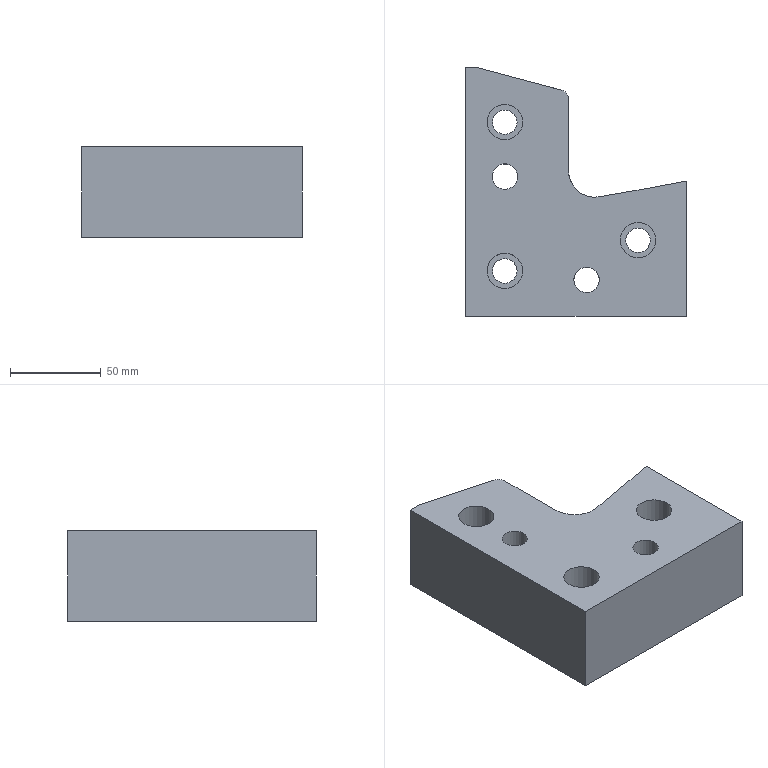Part | NX | features solid 2 | 1 solid | 23 faces | box 121.642 x 136.888 x 50 mm | volume 539772 mm3 | plane 11 | cylinder 10 | spline 2 | commonest cylinder face diameters 13.5 x3 19.5 x3 10 x2 14 x2
STEP:
#1=CARTESIAN_POINT('',(-1318.358,395.,0.));
#2=VERTEX_POINT('',#1);
#3=CARTESIAN_POINT('',(-1325.,395.,0.));
#4=VERTEX_POINT('',#3);
#5=CARTESIAN_POINT('',(-1253.358,395.,0.));
#6=DIRECTION('',(-1.,0.,0.));
#7=VECTOR('',#6,1000.);
#8=LINE('',#5,#7);
#9=EDGE_CURVE('',#2,#4,#8,.T.);
#10=ORIENTED_EDGE('',*,*,#9,.F.);
#11=CARTESIAN_POINT('',(-1318.358,395.,-50.));
#12=VERTEX_POINT('',#11);
#13=CARTESIAN_POINT('',(-1318.358,395.,-15.));
#14=DIRECTION('',(0.,0.,-1.));
#15=VECTOR('',#14,1000.);
#16=LINE('',#13,#15);
#17=EDGE_CURVE('',#2,#12,#16,.T.);
#18=ORIENTED_EDGE('',*,*,#17,.T.);
#19=CARTESIAN_POINT('',(-1325.,395.,-50.));
#20=VERTEX_POINT('',#19);
#21=CARTESIAN_POINT('',(-1021.9,395.,-50.));
#22=DIRECTION('',(1.,0.,0.));
#23=VECTOR('',#22,1000.);
#24=LINE('',#21,#23);
#25=EDGE_CURVE('',#12,#20,#24,.F.);
#26=ORIENTED_EDGE('',*,*,#25,.T.);
#27=CARTESIAN_POINT('',(-1325.,395.,-60.));
#28=DIRECTION('',(0.,0.,-1.));
#29=VECTOR('',#28,1000.);
#30=LINE('',#27,#29);
#31=EDGE_CURVE('',#4,#20,#30,.T.);
#32=ORIENTED_EDGE('',*,*,#31,.F.);
#33=EDGE_LOOP('',(#10,#18,#26,#32));
#34=FACE_BOUND('',#33,.T.);
#35=CARTESIAN_POINT('',(-1245.,395.,0.));
#36=DIRECTION('',(0.,1.,0.));
#37=DIRECTION('',(0.,0.,1.));
#38=AXIS2_PLACEMENT_3D('',#35,#36,#37);
#39=PLANE('',#38);
#40=ADVANCED_FACE('',(#34),#39,.T.);
#41=CARTESIAN_POINT('',(-1310.108,365.,-25.));
#42=VERTEX_POINT('',#41);
#43=CARTESIAN_POINT('',(-1303.358,365.,-25.));
#44=DIRECTION('',(0.,0.,-1.));
#45=DIRECTION('',(-1.,0.,0.));
#46=AXIS2_PLACEMENT_3D('',#43,#44,#45);
#47=CIRCLE('',#46,6.75);
#48=EDGE_CURVE('',#42,#42,#47,.T.);
#49=ORIENTED_EDGE('',*,*,#48,.T.);
#50=EDGE_LOOP('',(#49));
#51=FACE_BOUND('',#50,.T.);
#52=CARTESIAN_POINT('',(-1313.108,365.,-25.));
#53=VERTEX_POINT('',#52);
#54=CARTESIAN_POINT('',(-1303.358,365.,-25.));
#55=DIRECTION('',(0.,0.,-1.));
#56=DIRECTION('',(-1.,0.,0.));
#57=AXIS2_PLACEMENT_3D('',#54,#55,#56);
#58=CIRCLE('',#57,9.75);
#59=EDGE_CURVE('',#53,#53,#58,.T.);
#60=ORIENTED_EDGE('',*,*,#59,.F.);
#61=EDGE_LOOP('',(#60));
#62=FACE_BOUND('',#61,.T.);
#63=CARTESIAN_POINT('',(-1303.358,345.,-25.));
#64=DIRECTION('',(0.,0.,-1.));
#65=DIRECTION('',(-1.,0.,0.));
#66=AXIS2_PLACEMENT_3D('',#63,#64,#65);
#67=PLANE('',#66);
#68=ADVANCED_FACE('',(#51,#62),#67,.F.);
#69=CARTESIAN_POINT('',(-1310.108,283.112,-25.));
#70=VERTEX_POINT('',#69);
#71=CARTESIAN_POINT('',(-1303.358,283.112,-25.));
#72=DIRECTION('',(0.,0.,-1.));
#73=DIRECTION('',(-1.,0.,0.));
#74=AXIS2_PLACEMENT_3D('',#71,#72,#73);
#75=CIRCLE('',#74,6.75);
#76=EDGE_CURVE('',#70,#70,#75,.T.);
#77=ORIENTED_EDGE('',*,*,#76,.T.);
#78=EDGE_LOOP('',(#77));
#79=FACE_BOUND('',#78,.T.);
#80=CARTESIAN_POINT('',(-1313.108,283.112,-25.));
#81=VERTEX_POINT('',#80);
#82=CARTESIAN_POINT('',(-1303.358,283.112,-25.));
#83=DIRECTION('',(0.,0.,-1.));
#84=DIRECTION('',(-1.,0.,0.));
#85=AXIS2_PLACEMENT_3D('',#82,#83,#84);
#86=CIRCLE('',#85,9.75);
#87=EDGE_CURVE('',#81,#81,#86,.T.);
#88=ORIENTED_EDGE('',*,*,#87,.F.);
#89=EDGE_LOOP('',(#88));
#90=FACE_BOUND('',#89,.T.);
#91=CARTESIAN_POINT('',(-1288.358,283.112,-25.));
#92=DIRECTION('',(0.,0.,-1.));
#93=DIRECTION('',(-1.,0.,0.));
#94=AXIS2_PLACEMENT_3D('',#91,#92,#93);
#95=PLANE('',#94);
#96=ADVANCED_FACE('',(#79,#90),#95,.F.);
#97=CARTESIAN_POINT('',(-1236.75,300.,-25.));
#98=VERTEX_POINT('',#97);
#99=CARTESIAN_POINT('',(-1230.,300.,-25.));
#100=DIRECTION('',(0.,0.,-1.));
#101=DIRECTION('',(-1.,0.,0.));
#102=AXIS2_PLACEMENT_3D('',#99,#100,#101);
#103=CIRCLE('',#102,6.75);
#104=EDGE_CURVE('',#98,#98,#103,.T.);
#105=ORIENTED_EDGE('',*,*,#104,.T.);
#106=EDGE_LOOP('',(#105));
#107=FACE_BOUND('',#106,.T.);
#108=CARTESIAN_POINT('',(-1239.75,300.,-25.));
#109=VERTEX_POINT('',#108);
#110=CARTESIAN_POINT('',(-1230.,300.,-25.));
#111=DIRECTION('',(0.,0.,-1.));
#112=DIRECTION('',(-1.,0.,0.));
#113=AXIS2_PLACEMENT_3D('',#110,#111,#112);
#114=CIRCLE('',#113,9.75);
#115=EDGE_CURVE('',#109,#109,#114,.T.);
#116=ORIENTED_EDGE('',*,*,#115,.F.);
#117=EDGE_LOOP('',(#116));
#118=FACE_BOUND('',#117,.T.);
#119=CARTESIAN_POINT('',(-1230.,300.,-25.));
#120=DIRECTION('',(0.,0.,-1.));
#121=DIRECTION('',(-1.,0.,0.));
#122=AXIS2_PLACEMENT_3D('',#119,#120,#121);
#123=PLANE('',#122);
#124=ADVANCED_FACE('',(#107,#118),#123,.F.);
#125=CARTESIAN_POINT('',(-1310.108,365.,-50.));
#126=VERTEX_POINT('',#125);
#127=CARTESIAN_POINT('',(-1303.358,365.,-50.));
#128=DIRECTION('',(0.,0.,-1.));
#129=DIRECTION('',(-1.,0.,0.));
#130=AXIS2_PLACEMENT_3D('',#127,#128,#129);
#131=CIRCLE('',#130,6.75);
#132=EDGE_CURVE('',#126,#126,#131,.T.);
#133=ORIENTED_EDGE('',*,*,#132,.T.);
#134=EDGE_LOOP('',(#133));
#135=FACE_BOUND('',#134,.T.);
#136=ORIENTED_EDGE('',*,*,#48,.F.);
#137=EDGE_LOOP('',(#136));
#138=FACE_BOUND('',#137,.T.);
#139=CARTESIAN_POINT('',(-1303.358,365.,-50.));
#140=DIRECTION('',(0.,0.,-1.));
#141=DIRECTION('',(-1.,0.,0.));
#142=AXIS2_PLACEMENT_3D('',#139,#140,#141);
#143=CYLINDRICAL_SURFACE('',#142,6.75);
#144=ADVANCED_FACE('',(#135,#138),#143,.F.);
#145=CARTESIAN_POINT('',(-1310.108,283.112,-50.));
#146=VERTEX_POINT('',#145);
#147=CARTESIAN_POINT('',(-1303.358,283.112,-50.));
#148=DIRECTION('',(0.,0.,-1.));
#149=DIRECTION('',(-1.,0.,0.));
#150=AXIS2_PLACEMENT_3D('',#147,#148,#149);
#151=CIRCLE('',#150,6.75);
#152=EDGE_CURVE('',#146,#146,#151,.T.);
#153=ORIENTED_EDGE('',*,*,#152,.T.);
#154=EDGE_LOOP('',(#153));
#155=FACE_BOUND('',#154,.T.);
#156=ORIENTED_EDGE('',*,*,#76,.F.);
#157=EDGE_LOOP('',(#156));
#158=FACE_BOUND('',#157,.T.);
#159=CARTESIAN_POINT('',(-1303.358,283.112,-50.));
#160=DIRECTION('',(0.,0.,-1.));
#161=DIRECTION('',(-1.,0.,0.));
#162=AXIS2_PLACEMENT_3D('',#159,#160,#161);
#163=CYLINDRICAL_SURFACE('',#162,6.75);
#164=ADVANCED_FACE('',(#155,#158),#163,.F.);
#165=CARTESIAN_POINT('',(-1236.75,300.,-50.));
#166=VERTEX_POINT('',#165);
#167=CARTESIAN_POINT('',(-1230.,300.,-50.));
#168=DIRECTION('',(0.,0.,-1.));
#169=DIRECTION('',(-1.,0.,0.));
#170=AXIS2_PLACEMENT_3D('',#167,#168,#169);
#171=CIRCLE('',#170,6.75);
#172=EDGE_CURVE('',#166,#166,#171,.T.);
#173=ORIENTED_EDGE('',*,*,#172,.T.);
#174=EDGE_LOOP('',(#173));
#175=FACE_BOUND('',#174,.T.);
#176=ORIENTED_EDGE('',*,*,#104,.F.);
#177=EDGE_LOOP('',(#176));
#178=FACE_BOUND('',#177,.T.);
#179=CARTESIAN_POINT('',(-1230.,300.,-50.));
#180=DIRECTION('',(0.,0.,-1.));
#181=DIRECTION('',(-1.,0.,0.));
#182=AXIS2_PLACEMENT_3D('',#179,#180,#181);
#183=CYLINDRICAL_SURFACE('',#182,6.75);
#184=ADVANCED_FACE('',(#175,#178),#183,.F.);
#185=CARTESIAN_POINT('',(-1203.358,258.112,-50.));
#186=VERTEX_POINT('',#185);
#187=CARTESIAN_POINT('',(-1203.358,258.112,0.));
#188=VERTEX_POINT('',#187);
#189=CARTESIAN_POINT('',(-1203.358,258.112,-50.));
#190=DIRECTION('',(0.,0.,1.));
#191=VECTOR('',#190,1000.);
#192=LINE('',#189,#191);
#193=EDGE_CURVE('',#186,#188,#192,.T.);
#194=ORIENTED_EDGE('',*,*,#193,.T.);
#195=CARTESIAN_POINT('',(-1325.,258.112,0.));
#196=VERTEX_POINT('',#195);
#197=CARTESIAN_POINT('',(-1253.358,258.112,0.));
#198=DIRECTION('',(-1.,0.,0.));
#199=VECTOR('',#198,1000.);
#200=LINE('',#197,#199);
#201=EDGE_CURVE('',#188,#196,#200,.T.);
#202=ORIENTED_EDGE('',*,*,#201,.T.);
#203=CARTESIAN_POINT('',(-1325.,258.112,-50.));
#204=VERTEX_POINT('',#203);
#205=CARTESIAN_POINT('',(-1325.,258.112,-60.));
#206=DIRECTION('',(0.,0.,-1.));
#207=VECTOR('',#206,1000.);
#208=LINE('',#205,#207);
#209=EDGE_CURVE('',#196,#204,#208,.T.);
#210=ORIENTED_EDGE('',*,*,#209,.T.);
#211=CARTESIAN_POINT('',(-1021.9,258.112,-50.));
#212=DIRECTION('',(1.,0.,0.));
#213=VECTOR('',#212,1000.);
#214=LINE('',#211,#213);
#215=EDGE_CURVE('',#186,#204,#214,.F.);
#216=ORIENTED_EDGE('',*,*,#215,.F.);
#217=EDGE_LOOP('',(#194,#202,#210,#216));
#218=FACE_BOUND('',#217,.T.);
#219=CARTESIAN_POINT('',(-1203.358,258.112,0.));
#220=DIRECTION('',(0.,1.,0.));
#221=DIRECTION('',(0.,0.,1.));
#222=AXIS2_PLACEMENT_3D('',#219,#220,#221);
#223=PLANE('',#222);
#224=ADVANCED_FACE('',(#218),#223,.F.);
#225=CARTESIAN_POINT('',(-1265.358,278.112,-50.));
#226=VERTEX_POINT('',#225);
#227=CARTESIAN_POINT('',(-1258.358,278.112,-50.));
#228=DIRECTION('',(0.,0.,-1.));
#229=DIRECTION('',(-1.,0.,0.));
#230=AXIS2_PLACEMENT_3D('',#227,#228,#229);
#231=CIRCLE('',#230,7.);
#232=EDGE_CURVE('',#226,#226,#231,.T.);
#233=ORIENTED_EDGE('',*,*,#232,.T.);
#234=EDGE_LOOP('',(#233));
#235=FACE_BOUND('',#234,.T.);
#236=CARTESIAN_POINT('',(-1265.358,278.112,0.));
#237=VERTEX_POINT('',#236);
#238=CARTESIAN_POINT('',(-1258.358,278.112,0.));
#239=DIRECTION('',(0.,0.,-1.));
#240=DIRECTION('',(-1.,0.,0.));
#241=AXIS2_PLACEMENT_3D('',#238,#239,#240);
#242=CIRCLE('',#241,7.);
#243=EDGE_CURVE('',#237,#237,#242,.T.);
#244=ORIENTED_EDGE('',*,*,#243,.F.);
#245=EDGE_LOOP('',(#244));
#246=FACE_BOUND('',#245,.T.);
#247=CARTESIAN_POINT('',(-1258.358,278.112,0.));
#248=DIRECTION('',(0.,0.,-1.));
#249=DIRECTION('',(-1.,0.,0.));
#250=AXIS2_PLACEMENT_3D('',#247,#248,#249);
#251=CYLINDRICAL_SURFACE('',#250,7.);
#252=ADVANCED_FACE('',(#235,#246),#251,.F.);
#253=ORIENTED_EDGE('',*,*,#59,.T.);
#254=EDGE_LOOP('',(#253));
#255=FACE_BOUND('',#254,.T.);
#256=CARTESIAN_POINT('',(-1313.108,365.,0.));
#257=VERTEX_POINT('',#256);
#258=CARTESIAN_POINT('',(-1303.358,365.,0.));
#259=DIRECTION('',(0.,0.,-1.));
#260=DIRECTION('',(-1.,0.,0.));
#261=AXIS2_PLACEMENT_3D('',#258,#259,#260);
#262=CIRCLE('',#261,9.75);
#263=EDGE_CURVE('',#257,#257,#262,.T.);
#264=ORIENTED_EDGE('',*,*,#263,.F.);
#265=EDGE_LOOP('',(#264));
#266=FACE_BOUND('',#265,.T.);
#267=CARTESIAN_POINT('',(-1303.358,365.,0.));
#268=DIRECTION('',(0.,0.,-1.));
#269=DIRECTION('',(-1.,0.,0.));
#270=AXIS2_PLACEMENT_3D('',#267,#268,#269);
#271=CYLINDRICAL_SURFACE('',#270,9.75);
#272=ADVANCED_FACE('',(#255,#266),#271,.F.);
#273=ORIENTED_EDGE('',*,*,#87,.T.);
#274=EDGE_LOOP('',(#273));
#275=FACE_BOUND('',#274,.T.);
#276=CARTESIAN_POINT('',(-1313.108,283.112,0.));
#277=VERTEX_POINT('',#276);
#278=CARTESIAN_POINT('',(-1303.358,283.112,0.));
#279=DIRECTION('',(0.,0.,-1.));
#280=DIRECTION('',(-1.,0.,0.));
#281=AXIS2_PLACEMENT_3D('',#278,#279,#280);
#282=CIRCLE('',#281,9.75);
#283=EDGE_CURVE('',#277,#277,#282,.T.);
#284=ORIENTED_EDGE('',*,*,#283,.F.);
#285=EDGE_LOOP('',(#284));
#286=FACE_BOUND('',#285,.T.);
#287=CARTESIAN_POINT('',(-1303.358,283.112,0.));
#288=DIRECTION('',(0.,0.,-1.));
#289=DIRECTION('',(-1.,0.,0.));
#290=AXIS2_PLACEMENT_3D('',#287,#288,#289);
#291=CYLINDRICAL_SURFACE('',#290,9.75);
#292=ADVANCED_FACE('',(#275,#286),#291,.F.);
#293=ORIENTED_EDGE('',*,*,#115,.T.);
#294=EDGE_LOOP('',(#293));
#295=FACE_BOUND('',#294,.T.);
#296=CARTESIAN_POINT('',(-1239.75,300.,0.));
#297=VERTEX_POINT('',#296);
#298=CARTESIAN_POINT('',(-1230.,300.,0.));
#299=DIRECTION('',(0.,0.,-1.));
#300=DIRECTION('',(-1.,0.,0.));
#301=AXIS2_PLACEMENT_3D('',#298,#299,#300);
#302=CIRCLE('',#301,9.75);
#303=EDGE_CURVE('',#297,#297,#302,.T.);
#304=ORIENTED_EDGE('',*,*,#303,.F.);
#305=EDGE_LOOP('',(#304));
#306=FACE_BOUND('',#305,.T.);
#307=CARTESIAN_POINT('',(-1230.,300.,0.));
#308=DIRECTION('',(0.,0.,-1.));
#309=DIRECTION('',(-1.,0.,0.));
#310=AXIS2_PLACEMENT_3D('',#307,#308,#309);
#311=CYLINDRICAL_SURFACE('',#310,9.75);
#312=ADVANCED_FACE('',(#295,#306),#311,.F.);
#313=CARTESIAN_POINT('',(-1203.358,332.538,-15.));
#314=VERTEX_POINT('',#313);
#315=CARTESIAN_POINT('',(-1203.358,330.489,-15.));
#316=VERTEX_POINT('',#315);
#317=CARTESIAN_POINT('',(-1203.358,250.,-15.));
#318=DIRECTION('',(0.,1.,0.));
#319=VECTOR('',#318,1000.);
#320=LINE('',#317,#319);
#321=EDGE_CURVE('',#314,#316,#320,.F.);
#322=ORIENTED_EDGE('',*,*,#321,.F.);
#323=CARTESIAN_POINT('',(-1203.358,332.538,0.));
#324=VERTEX_POINT('',#323);
#325=CARTESIAN_POINT('',(-1203.358,332.538,-100.));
#326=DIRECTION('',(0.,0.,1.));
#327=VECTOR('',#326,1000.);
#328=LINE('',#325,#327);
#329=EDGE_CURVE('',#324,#314,#328,.F.);
#330=ORIENTED_EDGE('',*,*,#329,.F.);
#331=CARTESIAN_POINT('',(-1203.358,307.899,0.));
#332=DIRECTION('',(0.,-1.,0.));
#333=VECTOR('',#332,1000.);
#334=LINE('',#331,#333);
#335=EDGE_CURVE('',#324,#188,#334,.T.);
#336=ORIENTED_EDGE('',*,*,#335,.T.);
#337=ORIENTED_EDGE('',*,*,#193,.F.);
#338=CARTESIAN_POINT('',(-1203.358,330.489,-50.));
#339=VERTEX_POINT('',#338);
#340=CARTESIAN_POINT('',(-1203.358,307.899,-50.));
#341=DIRECTION('',(0.,-1.,0.));
#342=VECTOR('',#341,1000.);
#343=LINE('',#340,#342);
#344=EDGE_CURVE('',#339,#186,#343,.T.);
#345=ORIENTED_EDGE('',*,*,#344,.F.);
#346=CARTESIAN_POINT('',(-1203.358,330.489,-32.5));
#347=DIRECTION('',(0.,0.,1.));
#348=VECTOR('',#347,1000.);
#349=LINE('',#346,#348);
#350=EDGE_CURVE('',#339,#316,#349,.T.);
#351=ORIENTED_EDGE('',*,*,#350,.T.);
#352=EDGE_LOOP('',(#322,#330,#336,#337,#345,#351));
#353=FACE_BOUND('',#352,.T.);
#354=CARTESIAN_POINT('',(-1203.358,250.,0.));
#355=DIRECTION('',(1.,0.,0.));
#356=DIRECTION('',(0.,0.,-1.));
#357=AXIS2_PLACEMENT_3D('',#354,#355,#356);
#358=PLANE('',#357);
#359=ADVANCED_FACE('',(#353),#358,.T.);
#360=CARTESIAN_POINT('',(-1270.358,378.302,-50.));
#361=VERTEX_POINT('',#360);
#362=CARTESIAN_POINT('',(-1203.358,330.489,-50.));
#363=CARTESIAN_POINT('',(-1208.021,329.456,-50.));
#364=CARTESIAN_POINT('',(-1215.042,328.141,-50.));
#365=CARTESIAN_POINT('',(-1224.396,326.524,-50.));
#366=CARTESIAN_POINT('',(-1231.398,325.331,-50.));
#367=CARTESIAN_POINT('',(-1237.23,324.32,-50.));
#368=CARTESIAN_POINT('',(-1241.899,323.51,-50.));
#369=CARTESIAN_POINT('',(-1245.394,322.899,-50.));
#370=CARTESIAN_POINT('',(-1248.327,322.398,-50.));
#371=CARTESIAN_POINT('',(-1250.62,321.979,-50.));
#372=CARTESIAN_POINT('',(-1252.531,321.673,-50.));
#373=CARTESIAN_POINT('',(-1254.609,321.607,-50.));
#374=CARTESIAN_POINT('',(-1257.298,321.883,-50.));
#375=CARTESIAN_POINT('',(-1260.584,322.891,-50.));
#376=CARTESIAN_POINT('',(-1264.046,325.04,-50.));
#377=CARTESIAN_POINT('',(-1266.887,327.947,-50.));
#378=CARTESIAN_POINT('',(-1268.96,331.413,-50.));
#379=CARTESIAN_POINT('',(-1270.19,335.291,-50.));
#380=CARTESIAN_POINT('',(-1270.428,339.274,-50.));
#381=CARTESIAN_POINT('',(-1270.366,342.757,-50.));
#382=CARTESIAN_POINT('',(-1270.377,346.328,-50.));
#383=CARTESIAN_POINT('',(-1270.367,351.059,-50.));
#384=CARTESIAN_POINT('',(-1270.365,356.984,-50.));
#385=CARTESIAN_POINT('',(-1270.36,364.089,-50.));
#386=CARTESIAN_POINT('',(-1270.359,371.195,-50.));
#387=CARTESIAN_POINT('',(-1270.358,375.933,-50.));
#388=CARTESIAN_POINT('',(-1270.358,378.302,-50.));
#389=B_SPLINE_CURVE_WITH_KNOTS('',3,(#362,#363,#364,#365,#366,#367,#368,#369,#370,#371,#372,#373,#374,#375,#376,#377,#378,#379,#380,#381,#382,#383,#384,#385,#386,#387,#388),.UNSPECIFIED.,.F.,.F.,(4,1,1,1,1,1,1,1,1,1,1,1,1,1,1,1,1,1,1,1,1,1,1,1,4),(0.002675,0.08837,0.1312,0.1741,0.2169,0.2383,0.2598,0.2812,0.2919,0.3026,0.3133,0.324,0.3455,0.3669,0.3883,0.4097,0.4312,0.4526,0.474,0.4954,0.5169,0.5597,0.6026,0.6454,0.6883),.UNSPECIFIED.);
#390=EDGE_CURVE('',#339,#361,#389,.T.);
#391=ORIENTED_EDGE('',*,*,#390,.T.);
#392=CARTESIAN_POINT('',(-1270.358,378.302,-15.));
#393=VERTEX_POINT('',#392);
#394=CARTESIAN_POINT('',(-1270.358,378.302,-15.));
#395=CARTESIAN_POINT('',(-1270.358,378.302,-26.667));
#396=CARTESIAN_POINT('',(-1270.358,378.302,-38.333));
#397=CARTESIAN_POINT('',(-1270.358,378.302,-50.));
#398=B_SPLINE_CURVE_WITH_KNOTS('',3,(#394,#395,#396,#397),.UNSPECIFIED.,.F.,.F.,(4,4),(0.,1.),.UNSPECIFIED.);
#399=EDGE_CURVE('',#361,#393,#398,.F.);
#400=ORIENTED_EDGE('',*,*,#399,.T.);
#401=CARTESIAN_POINT('',(-1203.358,330.489,-15.));
#402=CARTESIAN_POINT('',(-1208.021,329.456,-15.));
#403=CARTESIAN_POINT('',(-1215.042,328.141,-15.));
#404=CARTESIAN_POINT('',(-1224.396,326.524,-15.));
#405=CARTESIAN_POINT('',(-1231.398,325.331,-15.));
#406=CARTESIAN_POINT('',(-1237.23,324.32,-15.));
#407=CARTESIAN_POINT('',(-1241.899,323.51,-15.));
#408=CARTESIAN_POINT('',(-1245.394,322.899,-15.));
#409=CARTESIAN_POINT('',(-1248.327,322.398,-15.));
#410=CARTESIAN_POINT('',(-1250.62,321.979,-15.));
#411=CARTESIAN_POINT('',(-1252.531,321.673,-15.));
#412=CARTESIAN_POINT('',(-1254.609,321.607,-15.));
#413=CARTESIAN_POINT('',(-1257.298,321.883,-15.));
#414=CARTESIAN_POINT('',(-1260.584,322.891,-15.));
#415=CARTESIAN_POINT('',(-1264.046,325.04,-15.));
#416=CARTESIAN_POINT('',(-1266.887,327.947,-15.));
#417=CARTESIAN_POINT('',(-1268.96,331.413,-15.));
#418=CARTESIAN_POINT('',(-1270.19,335.291,-15.));
#419=CARTESIAN_POINT('',(-1270.428,339.274,-15.));
#420=CARTESIAN_POINT('',(-1270.366,342.757,-15.));
#421=CARTESIAN_POINT('',(-1270.377,346.328,-15.));
#422=CARTESIAN_POINT('',(-1270.367,351.059,-15.));
#423=CARTESIAN_POINT('',(-1270.365,356.984,-15.));
#424=CARTESIAN_POINT('',(-1270.36,364.089,-15.));
#425=CARTESIAN_POINT('',(-1270.359,371.195,-15.));
#426=CARTESIAN_POINT('',(-1270.358,375.933,-15.));
#427=CARTESIAN_POINT('',(-1270.358,378.302,-15.));
#428=B_SPLINE_CURVE_WITH_KNOTS('',3,(#401,#402,#403,#404,#405,#406,#407,#408,#409,#410,#411,#412,#413,#414,#415,#416,#417,#418,#419,#420,#421,#422,#423,#424,#425,#426,#427),.UNSPECIFIED.,.F.,.F.,(4,1,1,1,1,1,1,1,1,1,1,1,1,1,1,1,1,1,1,1,1,1,1,1,4),(0.002675,0.08837,0.1312,0.1741,0.2169,0.2383,0.2598,0.2812,0.2919,0.3026,0.3133,0.324,0.3455,0.3669,0.3883,0.4097,0.4312,0.4526,0.474,0.4954,0.5169,0.5597,0.6026,0.6454,0.6883),.UNSPECIFIED.);
#429=EDGE_CURVE('',#316,#393,#428,.T.);
#430=ORIENTED_EDGE('',*,*,#429,.F.);
#431=ORIENTED_EDGE('',*,*,#350,.F.);
#432=EDGE_LOOP('',(#391,#400,#430,#431));
#433=FACE_BOUND('',#432,.T.);
#434=CARTESIAN_POINT('',(-1203.358,330.489,-50.));
#435=CARTESIAN_POINT('',(-1203.358,330.489,-15.));
#436=CARTESIAN_POINT('',(-1208.021,329.456,-50.));
#437=CARTESIAN_POINT('',(-1208.021,329.456,-15.));
#438=CARTESIAN_POINT('',(-1215.042,328.141,-50.));
#439=CARTESIAN_POINT('',(-1215.042,328.141,-15.));
#440=CARTESIAN_POINT('',(-1224.396,326.524,-50.));
#441=CARTESIAN_POINT('',(-1224.396,326.524,-15.));
#442=CARTESIAN_POINT('',(-1231.398,325.331,-50.));
#443=CARTESIAN_POINT('',(-1231.398,325.331,-15.));
#444=CARTESIAN_POINT('',(-1237.23,324.32,-50.));
#445=CARTESIAN_POINT('',(-1237.23,324.32,-15.));
#446=CARTESIAN_POINT('',(-1241.899,323.51,-50.));
#447=CARTESIAN_POINT('',(-1241.899,323.51,-15.));
#448=CARTESIAN_POINT('',(-1245.394,322.899,-50.));
#449=CARTESIAN_POINT('',(-1245.394,322.899,-15.));
#450=CARTESIAN_POINT('',(-1248.327,322.398,-50.));
#451=CARTESIAN_POINT('',(-1248.327,322.398,-15.));
#452=CARTESIAN_POINT('',(-1250.62,321.979,-50.));
#453=CARTESIAN_POINT('',(-1250.62,321.979,-15.));
#454=CARTESIAN_POINT('',(-1252.531,321.673,-50.));
#455=CARTESIAN_POINT('',(-1252.531,321.673,-15.));
#456=CARTESIAN_POINT('',(-1254.609,321.607,-50.));
#457=CARTESIAN_POINT('',(-1254.609,321.607,-15.));
#458=CARTESIAN_POINT('',(-1257.298,321.883,-50.));
#459=CARTESIAN_POINT('',(-1257.298,321.883,-15.));
#460=CARTESIAN_POINT('',(-1260.584,322.891,-50.));
#461=CARTESIAN_POINT('',(-1260.584,322.891,-15.));
#462=CARTESIAN_POINT('',(-1264.046,325.04,-50.));
#463=CARTESIAN_POINT('',(-1264.046,325.04,-15.));
#464=CARTESIAN_POINT('',(-1266.887,327.947,-50.));
#465=CARTESIAN_POINT('',(-1266.887,327.947,-15.));
#466=CARTESIAN_POINT('',(-1268.96,331.413,-50.));
#467=CARTESIAN_POINT('',(-1268.96,331.413,-15.));
#468=CARTESIAN_POINT('',(-1270.19,335.291,-50.));
#469=CARTESIAN_POINT('',(-1270.19,335.291,-15.));
#470=CARTESIAN_POINT('',(-1270.428,339.274,-50.));
#471=CARTESIAN_POINT('',(-1270.428,339.274,-15.));
#472=CARTESIAN_POINT('',(-1270.366,342.757,-50.));
#473=CARTESIAN_POINT('',(-1270.366,342.757,-15.));
#474=CARTESIAN_POINT('',(-1270.377,346.328,-50.));
#475=CARTESIAN_POINT('',(-1270.377,346.328,-15.));
#476=CARTESIAN_POINT('',(-1270.367,351.059,-50.));
#477=CARTESIAN_POINT('',(-1270.367,351.059,-15.));
#478=CARTESIAN_POINT('',(-1270.365,356.984,-50.));
#479=CARTESIAN_POINT('',(-1270.365,356.984,-15.));
#480=CARTESIAN_POINT('',(-1270.36,364.089,-50.));
#481=CARTESIAN_POINT('',(-1270.36,364.089,-15.));
#482=CARTESIAN_POINT('',(-1270.359,371.195,-50.));
#483=CARTESIAN_POINT('',(-1270.359,371.195,-15.));
#484=CARTESIAN_POINT('',(-1270.358,375.933,-50.));
#485=CARTESIAN_POINT('',(-1270.358,375.933,-15.));
#486=CARTESIAN_POINT('',(-1270.358,378.302,-50.));
#487=CARTESIAN_POINT('',(-1270.358,378.302,-15.));
#488=B_SPLINE_SURFACE_WITH_KNOTS('',3,1,((#434,#435),(#436,#437),(#438,#439),(#440,#441),(#442,#443),(#444,#445),(#446,#447),(#448,#449),(#450,#451),(#452,#453),(#454,#455),(#456,#457),(#458,#459),(#460,#461),(#462,#463),(#464,#465),(#466,#467),(#468,#469),(#470,#471),(#472,#473),(#474,#475),(#476,#477),(#478,#479),(#480,#481),(#482,#483),(#484,#485),(#486,#487)),.SURF_OF_LINEAR_EXTRUSION.,.F.,.F.,.F.,(4,1,1,1,1,1,1,1,1,1,1,1,1,1,1,1,1,1,1,1,1,1,1,1,4),(2,2),(0.002675,0.08837,0.1312,0.1741,0.2169,0.2383,0.2598,0.2812,0.2919,0.3026,0.3133,0.324,0.3455,0.3669,0.3883,0.4097,0.4312,0.4526,0.474,0.4954,0.5169,0.5597,0.6026,0.6454,0.6883),(0.,1.),.UNSPECIFIED.);
#489=ADVANCED_FACE('',(#433),#488,.T.);
#490=CARTESIAN_POINT('',(-1274.064,383.131,-15.));
#491=VERTEX_POINT('',#490);
#492=CARTESIAN_POINT('',(-1272.064,382.595,-15.));
#493=VERTEX_POINT('',#492);
#494=CARTESIAN_POINT('',(-1318.358,395.,-15.));
#495=DIRECTION('',(-0.9659,0.2588,0.));
#496=VECTOR('',#495,1000.);
#497=LINE('',#494,#496);
#498=EDGE_CURVE('',#491,#493,#497,.F.);
#499=ORIENTED_EDGE('',*,*,#498,.T.);
#500=CARTESIAN_POINT('',(-1268.358,377.766,-15.));
#501=VERTEX_POINT('',#500);
#502=CARTESIAN_POINT('',(-1273.358,377.766,-15.));
#503=DIRECTION('',(0.,0.,-1.));
#504=DIRECTION('',(-1.,0.,0.));
#505=AXIS2_PLACEMENT_3D('',#502,#503,#504);
#506=CIRCLE('',#505,5.);
#507=EDGE_CURVE('',#493,#501,#506,.T.);
#508=ORIENTED_EDGE('',*,*,#507,.T.);
#509=CARTESIAN_POINT('',(-169.554,563.744,-15.));
#510=CARTESIAN_POINT('',(-255.297,544.568,-15.));
#511=CARTESIAN_POINT('',(-341.04,525.392,-15.));
#512=CARTESIAN_POINT('',(-426.783,506.216,-15.));
#513=CARTESIAN_POINT('',(-492.739,491.465,-15.));
#514=CARTESIAN_POINT('',(-558.696,476.715,-15.));
#515=CARTESIAN_POINT('',(-624.652,461.964,-15.));
#516=CARTESIAN_POINT('',(-675.387,450.617,-15.));
#517=CARTESIAN_POINT('',(-726.123,439.27,-15.));
#518=CARTESIAN_POINT('',(-776.858,427.923,-15.));
#519=CARTESIAN_POINT('',(-815.885,419.195,-15.));
#520=CARTESIAN_POINT('',(-854.913,410.467,-15.));
#521=CARTESIAN_POINT('',(-893.94,401.738,-15.));
#522=CARTESIAN_POINT('',(-923.961,395.024,-15.));
#523=CARTESIAN_POINT('',(-953.982,388.31,-15.));
#524=CARTESIAN_POINT('',(-984.003,381.596,-15.));
#525=CARTESIAN_POINT('',(-1007.096,376.432,-15.));
#526=CARTESIAN_POINT('',(-1030.189,371.267,-15.));
#527=CARTESIAN_POINT('',(-1053.282,366.102,-15.));
#528=CARTESIAN_POINT('',(-1071.046,362.129,-15.));
#529=CARTESIAN_POINT('',(-1088.81,358.157,-15.));
#530=CARTESIAN_POINT('',(-1106.574,354.184,-15.));
#531=CARTESIAN_POINT('',(-1120.238,351.128,-15.));
#532=CARTESIAN_POINT('',(-1133.903,348.072,-15.));
#533=CARTESIAN_POINT('',(-1147.568,345.016,-15.));
#534=CARTESIAN_POINT('',(-1158.079,342.665,-15.));
#535=CARTESIAN_POINT('',(-1168.59,340.314,-15.));
#536=CARTESIAN_POINT('',(-1179.101,337.963,-15.));
#537=CARTESIAN_POINT('',(-1187.187,336.155,-15.));
#538=CARTESIAN_POINT('',(-1195.272,334.347,-15.));
#539=CARTESIAN_POINT('',(-1203.358,332.538,-15.));
#540=CARTESIAN_POINT('',(-1203.741,332.453,-15.));
#541=CARTESIAN_POINT('',(-1207.014,331.73,-15.));
#542=CARTESIAN_POINT('',(-1215.576,330.046,-15.));
#543=CARTESIAN_POINT('',(-1229.105,327.764,-15.));
#544=CARTESIAN_POINT('',(-1240.809,325.729,-15.));
#545=CARTESIAN_POINT('',(-1247.768,324.519,-15.));
#546=CARTESIAN_POINT('',(-1249.983,324.133,-15.));
#547=CARTESIAN_POINT('',(-1251.61,323.834,-15.));
#548=CARTESIAN_POINT('',(-1253.223,323.633,-15.));
#549=CARTESIAN_POINT('',(-1255.35,323.635,-15.));
#550=CARTESIAN_POINT('',(-1259.031,324.277,-15.));
#551=CARTESIAN_POINT('',(-1263.737,327.014,-15.));
#552=CARTESIAN_POINT('',(-1266.869,331.442,-15.));
#553=CARTESIAN_POINT('',(-1268.142,335.513,-15.));
#554=CARTESIAN_POINT('',(-1268.384,338.163,-15.));
#555=CARTESIAN_POINT('',(-1268.358,356.108,-15.));
#556=CARTESIAN_POINT('',(-1268.358,386.543,-15.));
#557=CARTESIAN_POINT('',(-1268.358,416.449,-15.));
#558=CARTESIAN_POINT('',(-1268.358,430.,-15.));
#559=CARTESIAN_POINT('',(-1268.358,438.292,-15.));
#560=CARTESIAN_POINT('',(-1268.358,446.585,-15.));
#561=CARTESIAN_POINT('',(-1268.358,454.877,-15.));
#562=CARTESIAN_POINT('',(-1268.358,465.657,-15.));
#563=CARTESIAN_POINT('',(-1268.358,476.437,-15.));
#564=CARTESIAN_POINT('',(-1268.358,487.217,-15.));
#565=CARTESIAN_POINT('',(-1268.358,501.231,-15.));
#566=CARTESIAN_POINT('',(-1268.358,515.245,-15.));
#567=CARTESIAN_POINT('',(-1268.358,529.259,-15.));
#568=CARTESIAN_POINT('',(-1268.358,547.477,-15.));
#569=CARTESIAN_POINT('',(-1268.358,565.695,-15.));
#570=CARTESIAN_POINT('',(-1268.358,583.913,-15.));
#571=CARTESIAN_POINT('',(-1268.358,607.597,-15.));
#572=CARTESIAN_POINT('',(-1268.358,631.281,-15.));
#573=CARTESIAN_POINT('',(-1268.358,654.964,-15.));
#574=CARTESIAN_POINT('',(-1268.358,685.753,-15.));
#575=CARTESIAN_POINT('',(-1268.358,716.542,-15.));
#576=CARTESIAN_POINT('',(-1268.358,747.33,-15.));
#577=CARTESIAN_POINT('',(-1268.358,787.356,-15.));
#578=CARTESIAN_POINT('',(-1268.358,827.381,-15.));
#579=CARTESIAN_POINT('',(-1268.358,867.406,-15.));
#580=CARTESIAN_POINT('',(-1268.358,919.439,-15.));
#581=CARTESIAN_POINT('',(-1268.358,971.472,-15.));
#582=CARTESIAN_POINT('',(-1268.358,1023.505,-15.));
#583=CARTESIAN_POINT('',(-1268.358,1091.148,-15.));
#584=CARTESIAN_POINT('',(-1268.358,1158.791,-15.));
#585=CARTESIAN_POINT('',(-1268.358,1226.434,-15.));
#586=CARTESIAN_POINT('',(-1268.358,1314.37,-15.));
#587=CARTESIAN_POINT('',(-1268.358,1402.305,-15.));
#588=CARTESIAN_POINT('',(-1268.358,1490.241,-15.));
#589=B_SPLINE_CURVE_WITH_KNOTS('',3,(#509,#510,#511,#512,#513,#514,#515,#516,#517,#518,#519,#520,#521,#522,#523,#524,#525,#526,#527,#528,#529,#530,#531,#532,#533,#534,#535,#536,#537,#538,#539,#540,#541,#542,#543,#544,#545,#546,#547,#548,#549,#550,#551,#552,#553,#554,#555,#556,#557,#558,#559,#560,#561,#562,#563,#564,#565,#566,#567,#568,#569,#570,#571,#572,#573,#574,#575,#576,#577,#578,#579,#580,#581,#582,#583,#584,#585,#586,#587,#588),.UNSPECIFIED.,.F.,.F.,(4,3,3,3,3,3,3,3,3,3,3,1,1,1,1,1,1,1,1,1,1,1,1,1,1,1,1,3,3,3,3,3,3,3,3,3,3,4),(-6.393,-4.802,-3.579,-2.637,-1.913,-1.356,-0.9281,-0.5985,-0.345,-0.15,0.,0.007116,0.06068,0.158,0.2552,0.2756,0.2857,0.2959,0.3055,0.3151,0.3343,0.3727,0.4111,0.4303,0.4495,0.459,0.7549,1.,1.15,1.345,1.599,1.928,2.356,2.913,3.637,4.579,5.802,7.393),.UNSPECIFIED.);
#590=EDGE_CURVE('',#314,#501,#589,.T.);
#591=ORIENTED_EDGE('',*,*,#590,.F.);
#592=ORIENTED_EDGE('',*,*,#321,.T.);
#593=ORIENTED_EDGE('',*,*,#429,.T.);
#594=CARTESIAN_POINT('',(-1275.358,378.302,-15.));
#595=DIRECTION('',(0.,0.,-1.));
#596=DIRECTION('',(-1.,0.,0.));
#597=AXIS2_PLACEMENT_3D('',#594,#595,#596);
#598=CIRCLE('',#597,5.);
#599=EDGE_CURVE('',#393,#491,#598,.F.);
#600=ORIENTED_EDGE('',*,*,#599,.T.);
#601=EDGE_LOOP('',(#499,#508,#591,#592,#593,#600));
#602=FACE_BOUND('',#601,.T.);
#603=CARTESIAN_POINT('',(-1203.358,332.538,-15.));
#604=DIRECTION('',(0.,0.,-1.));
#605=DIRECTION('',(-1.,0.,0.));
#606=AXIS2_PLACEMENT_3D('',#603,#604,#605);
#607=PLANE('',#606);
#608=ADVANCED_FACE('',(#602),#607,.T.);
#609=CARTESIAN_POINT('',(-1310.358,335.,0.));
#610=VERTEX_POINT('',#609);
#611=CARTESIAN_POINT('',(-1303.358,335.,0.));
#612=DIRECTION('',(0.,0.,-1.));
#613=DIRECTION('',(-1.,0.,0.));
#614=AXIS2_PLACEMENT_3D('',#611,#612,#613);
#615=CIRCLE('',#614,7.);
#616=EDGE_CURVE('',#610,#610,#615,.T.);
#617=ORIENTED_EDGE('',*,*,#616,.T.);
#618=EDGE_LOOP('',(#617));
#619=FACE_BOUND('',#618,.T.);
#620=ORIENTED_EDGE('',*,*,#303,.T.);
#621=EDGE_LOOP('',(#620));
#622=FACE_BOUND('',#621,.T.);
#623=ORIENTED_EDGE('',*,*,#283,.T.);
#624=EDGE_LOOP('',(#623));
#625=FACE_BOUND('',#624,.T.);
#626=ORIENTED_EDGE('',*,*,#263,.T.);
#627=EDGE_LOOP('',(#626));
#628=FACE_BOUND('',#627,.T.);
#629=ORIENTED_EDGE('',*,*,#243,.T.);
#630=EDGE_LOOP('',(#629));
#631=FACE_BOUND('',#630,.T.);
#632=CARTESIAN_POINT('',(-1268.358,377.766,0.));
#633=VERTEX_POINT('',#632);
#634=CARTESIAN_POINT('',(-1268.358,3406.296,0.));
#635=CARTESIAN_POINT('',(-1268.358,3160.274,0.));
#636=CARTESIAN_POINT('',(-1268.358,2914.251,0.));
#637=CARTESIAN_POINT('',(-1268.358,2668.228,0.));
#638=CARTESIAN_POINT('',(-1268.358,2478.98,0.));
#639=CARTESIAN_POINT('',(-1268.358,2289.732,0.));
#640=CARTESIAN_POINT('',(-1268.358,2100.484,0.));
#641=CARTESIAN_POINT('',(-1268.358,1954.908,0.));
#642=CARTESIAN_POINT('',(-1268.358,1809.333,0.));
#643=CARTESIAN_POINT('',(-1268.358,1663.757,0.));
#644=CARTESIAN_POINT('',(-1268.358,1551.776,0.));
#645=CARTESIAN_POINT('',(-1268.358,1439.795,0.));
#646=CARTESIAN_POINT('',(-1268.358,1327.814,0.));
#647=CARTESIAN_POINT('',(-1268.358,1241.674,0.));
#648=CARTESIAN_POINT('',(-1268.358,1155.535,0.));
#649=CARTESIAN_POINT('',(-1268.358,1069.395,0.));
#650=CARTESIAN_POINT('',(-1268.358,1003.134,0.));
#651=CARTESIAN_POINT('',(-1268.358,936.873,0.));
#652=CARTESIAN_POINT('',(-1268.358,870.612,0.));
#653=CARTESIAN_POINT('',(-1268.358,819.642,0.));
#654=CARTESIAN_POINT('',(-1268.358,768.672,0.));
#655=CARTESIAN_POINT('',(-1268.358,717.702,0.));
#656=CARTESIAN_POINT('',(-1268.358,678.494,0.));
#657=CARTESIAN_POINT('',(-1268.358,639.287,0.));
#658=CARTESIAN_POINT('',(-1268.358,600.079,0.));
#659=CARTESIAN_POINT('',(-1268.358,569.919,0.));
#660=CARTESIAN_POINT('',(-1268.358,539.759,0.));
#661=CARTESIAN_POINT('',(-1268.358,509.6,0.));
#662=CARTESIAN_POINT('',(-1268.358,486.4,0.));
#663=CARTESIAN_POINT('',(-1268.358,463.2,0.));
#664=CARTESIAN_POINT('',(-1268.358,440.,0.));
#665=CARTESIAN_POINT('',(-1268.358,423.116,0.));
#666=CARTESIAN_POINT('',(-1268.358,389.876,0.));
#667=CARTESIAN_POINT('',(-1268.358,356.108,0.));
#668=CARTESIAN_POINT('',(-1268.384,338.163,0.));
#669=CARTESIAN_POINT('',(-1268.142,335.513,0.));
#670=CARTESIAN_POINT('',(-1266.869,331.442,0.));
#671=CARTESIAN_POINT('',(-1263.737,327.014,0.));
#672=CARTESIAN_POINT('',(-1259.031,324.277,0.));
#673=CARTESIAN_POINT('',(-1255.35,323.635,0.));
#674=CARTESIAN_POINT('',(-1253.223,323.633,0.));
#675=CARTESIAN_POINT('',(-1251.61,323.834,0.));
#676=CARTESIAN_POINT('',(-1249.983,324.133,0.));
#677=CARTESIAN_POINT('',(-1247.768,324.519,0.));
#678=CARTESIAN_POINT('',(-1240.809,325.729,0.));
#679=CARTESIAN_POINT('',(-1229.105,327.764,0.));
#680=CARTESIAN_POINT('',(-1215.576,330.046,0.));
#681=CARTESIAN_POINT('',(-1198.69,333.366,0.));
#682=CARTESIAN_POINT('',(-1181.579,338.217,0.));
#683=CARTESIAN_POINT('',(-1161.617,343.876,0.));
#684=CARTESIAN_POINT('',(-1147.182,347.09,0.));
#685=CARTESIAN_POINT('',(-1132.006,349.651,0.));
#686=CARTESIAN_POINT('',(-1113.357,352.894,0.));
#687=CARTESIAN_POINT('',(-1078.972,358.874,0.));
#688=CARTESIAN_POINT('',(-1041.673,365.361,0.));
#689=CARTESIAN_POINT('',(-1004.375,371.848,0.));
#690=CARTESIAN_POINT('',(-976.401,376.715,0.));
#691=CARTESIAN_POINT('',(-948.425,381.569,0.));
#692=CARTESIAN_POINT('',(-929.78,384.838,0.));
#693=CARTESIAN_POINT('',(-920.448,386.415,0.));
#694=CARTESIAN_POINT('',(-897.572,390.281,0.));
#695=CARTESIAN_POINT('',(-874.697,394.148,0.));
#696=CARTESIAN_POINT('',(-851.821,398.014,0.));
#697=CARTESIAN_POINT('',(-822.083,403.041,0.));
#698=CARTESIAN_POINT('',(-792.345,408.067,0.));
#699=CARTESIAN_POINT('',(-762.607,413.094,0.));
#700=CARTESIAN_POINT('',(-723.948,419.628,0.));
#701=CARTESIAN_POINT('',(-685.289,426.162,0.));
#702=CARTESIAN_POINT('',(-646.629,432.697,0.));
#703=CARTESIAN_POINT('',(-596.372,441.191,0.));
#704=CARTESIAN_POINT('',(-546.115,449.686,0.));
#705=CARTESIAN_POINT('',(-495.858,458.181,0.));
#706=CARTESIAN_POINT('',(-430.523,469.224,0.));
#707=CARTESIAN_POINT('',(-365.189,480.267,0.));
#708=CARTESIAN_POINT('',(-299.855,491.31,0.));
#709=CARTESIAN_POINT('',(-214.92,505.666,0.));
#710=CARTESIAN_POINT('',(-129.985,520.022,0.));
#711=CARTESIAN_POINT('',(-45.051,534.378,0.));
#712=CARTESIAN_POINT('',(65.364,553.041,0.));
#713=CARTESIAN_POINT('',(175.78,571.703,0.));
#714=CARTESIAN_POINT('',(286.195,590.366,0.));
#715=CARTESIAN_POINT('',(429.734,614.628,0.));
#716=CARTESIAN_POINT('',(573.274,638.889,0.));
#717=CARTESIAN_POINT('',(716.813,663.151,0.));
#718=CARTESIAN_POINT('',(903.415,694.691,0.));
#719=CARTESIAN_POINT('',(1090.016,726.231,0.));
#720=CARTESIAN_POINT('',(1276.618,757.771,0.));
#721=CARTESIAN_POINT('',(1519.2,798.773,0.));
#722=CARTESIAN_POINT('',(1761.782,839.775,0.));
#723=CARTESIAN_POINT('',(2004.364,880.777,0.));
#724=B_SPLINE_CURVE_WITH_KNOTS('',3,(#634,#635,#636,#637,#638,#639,#640,#641,#642,#643,#644,#645,#646,#647,#648,#649,#650,#651,#652,#653,#654,#655,#656,#657,#658,#659,#660,#661,#662,#663,#664,#665,#666,#667,#668,#669,#670,#671,#672,#673,#674,#675,#676,#677,#678,#679,#680,#681,#682,#683,#684,#685,#686,#687,#688,#689,#690,#691,#692,#693,#694,#695,#696,#697,#698,#699,#700,#701,#702,#703,#704,#705,#706,#707,#708,#709,#710,#711,#712,#713,#714,#715,#716,#717,#718,#719,#720,#721,#722,#723),.UNSPECIFIED.,.F.,.F.,(4,3,3,3,3,3,3,3,3,3,3,1,1,1,1,1,1,1,1,1,1,1,1,1,1,1,1,1,1,1,1,1,1,1,1,1,1,3,3,3,3,3,3,3,3,3,3,4),(-6.393,-4.802,-3.579,-2.637,-1.913,-1.356,-0.9281,-0.5985,-0.345,-0.15,0.,0.1092,0.2149,0.2183,0.2252,0.2321,0.2458,0.2595,0.2664,0.2698,0.2732,0.2769,0.2805,0.2878,0.3225,0.3573,0.3764,0.4339,0.4722,0.5104,0.5296,0.5716,0.6328,0.7552,0.8164,0.8776,0.9388,1.,1.15,1.345,1.599,1.928,2.356,2.913,3.637,4.579,5.802,7.393),.UNSPECIFIED.);
#725=EDGE_CURVE('',#633,#324,#724,.T.);
#726=ORIENTED_EDGE('',*,*,#725,.F.);
#727=CARTESIAN_POINT('',(-1272.064,382.595,0.));
#728=VERTEX_POINT('',#727);
#729=CARTESIAN_POINT('',(-1273.358,377.766,0.));
#730=DIRECTION('',(0.,0.,1.));
#731=DIRECTION('',(1.,0.,0.));
#732=AXIS2_PLACEMENT_3D('',#729,#730,#731);
#733=CIRCLE('',#732,5.);
#734=EDGE_CURVE('',#633,#728,#733,.T.);
#735=ORIENTED_EDGE('',*,*,#734,.T.);
#736=CARTESIAN_POINT('',(-1242.386,374.643,0.));
#737=DIRECTION('',(-0.9659,0.2588,0.));
#738=VECTOR('',#737,1000.);
#739=LINE('',#736,#738);
#740=EDGE_CURVE('',#728,#2,#739,.T.);
#741=ORIENTED_EDGE('',*,*,#740,.T.);
#742=ORIENTED_EDGE('',*,*,#9,.T.);
#743=CARTESIAN_POINT('',(-1325.,338.697,0.));
#744=DIRECTION('',(0.,-1.,0.));
#745=VECTOR('',#744,1000.);
#746=LINE('',#743,#745);
#747=EDGE_CURVE('',#4,#196,#746,.T.);
#748=ORIENTED_EDGE('',*,*,#747,.T.);
#749=ORIENTED_EDGE('',*,*,#201,.F.);
#750=ORIENTED_EDGE('',*,*,#335,.F.);
#751=EDGE_LOOP('',(#726,#735,#741,#742,#748,#749,#750));
#752=FACE_BOUND('',#751,.T.);
#753=CARTESIAN_POINT('',(-1253.358,338.697,0.));
#754=DIRECTION('',(0.,0.,1.));
#755=DIRECTION('',(1.,0.,0.));
#756=AXIS2_PLACEMENT_3D('',#753,#754,#755);
#757=PLANE('',#756);
#758=ADVANCED_FACE('',(#619,#622,#625,#628,#631,#752),#757,.T.);
#759=ORIENTED_EDGE('',*,*,#747,.F.);
#760=ORIENTED_EDGE('',*,*,#31,.T.);
#761=CARTESIAN_POINT('',(-1325.,307.899,-50.));
#762=DIRECTION('',(0.,1.,0.));
#763=VECTOR('',#762,1000.);
#764=LINE('',#761,#763);
#765=EDGE_CURVE('',#20,#204,#764,.F.);
#766=ORIENTED_EDGE('',*,*,#765,.T.);
#767=ORIENTED_EDGE('',*,*,#209,.F.);
#768=EDGE_LOOP('',(#759,#760,#766,#767));
#769=FACE_BOUND('',#768,.T.);
#770=CARTESIAN_POINT('',(-1325.,430.,-60.));
#771=DIRECTION('',(-1.,0.,0.));
#772=DIRECTION('',(0.,-1.,0.));
#773=AXIS2_PLACEMENT_3D('',#770,#771,#772);
#774=PLANE('',#773);
#775=ADVANCED_FACE('',(#769),#774,.T.);
#776=ORIENTED_EDGE('',*,*,#590,.T.);
#777=CARTESIAN_POINT('',(-1268.358,377.766,0.));
#778=CARTESIAN_POINT('',(-1268.358,377.766,-5.));
#779=CARTESIAN_POINT('',(-1268.358,377.766,-10.));
#780=CARTESIAN_POINT('',(-1268.358,377.766,-15.));
#781=B_SPLINE_CURVE_WITH_KNOTS('',3,(#777,#778,#779,#780),.UNSPECIFIED.,.F.,.F.,(4,4),(0.,1.),.UNSPECIFIED.);
#782=EDGE_CURVE('',#501,#633,#781,.F.);
#783=ORIENTED_EDGE('',*,*,#782,.T.);
#784=ORIENTED_EDGE('',*,*,#725,.T.);
#785=ORIENTED_EDGE('',*,*,#329,.T.);
#786=EDGE_LOOP('',(#776,#783,#784,#785));
#787=FACE_BOUND('',#786,.T.);
#788=CARTESIAN_POINT('',(-1268.358,377.766,-15.));
#789=CARTESIAN_POINT('',(-1268.358,377.766,0.));
#790=CARTESIAN_POINT('',(-1268.358,375.399,-15.));
#791=CARTESIAN_POINT('',(-1268.358,375.399,0.));
#792=CARTESIAN_POINT('',(-1268.359,370.665,-15.));
#793=CARTESIAN_POINT('',(-1268.359,370.665,0.));
#794=CARTESIAN_POINT('',(-1268.362,363.564,-15.));
#795=CARTESIAN_POINT('',(-1268.362,363.564,0.));
#796=CARTESIAN_POINT('',(-1268.362,356.465,-15.));
#797=CARTESIAN_POINT('',(-1268.362,356.465,0.));
#798=CARTESIAN_POINT('',(-1268.38,349.357,-15.));
#799=CARTESIAN_POINT('',(-1268.38,349.357,0.));
#800=CARTESIAN_POINT('',(-1268.341,342.282,-15.));
#801=CARTESIAN_POINT('',(-1268.341,342.282,0.));
#802=CARTESIAN_POINT('',(-1268.527,335.088,-15.));
#803=CARTESIAN_POINT('',(-1268.527,335.088,0.));
#804=CARTESIAN_POINT('',(-1265.301,328.509,-15.));
#805=CARTESIAN_POINT('',(-1265.301,328.509,0.));
#806=CARTESIAN_POINT('',(-1260.437,324.845,-15.));
#807=CARTESIAN_POINT('',(-1260.437,324.845,0.));
#808=CARTESIAN_POINT('',(-1255.829,323.594,-15.));
#809=CARTESIAN_POINT('',(-1255.829,323.594,0.));
#810=CARTESIAN_POINT('',(-1252.254,323.645,-15.));
#811=CARTESIAN_POINT('',(-1252.254,323.645,0.));
#812=CARTESIAN_POINT('',(-1248.771,324.369,-15.));
#813=CARTESIAN_POINT('',(-1248.771,324.369,0.));
#814=CARTESIAN_POINT('',(-1245.269,324.946,-15.));
#815=CARTESIAN_POINT('',(-1245.269,324.946,0.));
#816=CARTESIAN_POINT('',(-1241.772,325.563,-15.));
#817=CARTESIAN_POINT('',(-1241.772,325.563,0.));
#818=CARTESIAN_POINT('',(-1237.108,326.37,-15.));
#819=CARTESIAN_POINT('',(-1237.108,326.37,0.));
#820=CARTESIAN_POINT('',(-1228.945,327.786,-15.));
#821=CARTESIAN_POINT('',(-1228.945,327.786,0.));
#822=CARTESIAN_POINT('',(-1217.272,329.752,-15.));
#823=CARTESIAN_POINT('',(-1217.272,329.752,0.));
#824=CARTESIAN_POINT('',(-1207.973,331.506,-15.));
#825=CARTESIAN_POINT('',(-1207.973,331.506,0.));
#826=CARTESIAN_POINT('',(-1203.358,332.538,-15.));
#827=CARTESIAN_POINT('',(-1203.358,332.538,0.));
#828=B_SPLINE_SURFACE_WITH_KNOTS('',3,1,((#788,#789),(#790,#791),(#792,#793),(#794,#795),(#796,#797),(#798,#799),(#800,#801),(#802,#803),(#804,#805),(#806,#807),(#808,#809),(#810,#811),(#812,#813),(#814,#815),(#816,#817),(#818,#819),(#820,#821),(#822,#823),(#824,#825),(#826,#827)),.SURF_OF_LINEAR_EXTRUSION.,.F.,.F.,.F.,(4,1,1,1,1,1,1,1,1,1,1,1,1,1,1,1,1,4),(2,2),(0.1341,0.1494,0.1647,0.18,0.1953,0.2106,0.2259,0.2413,0.2566,0.2642,0.2719,0.2795,0.2872,0.2948,0.3025,0.3178,0.3484,0.379),(0.,1.),.UNSPECIFIED.);
#829=ADVANCED_FACE('',(#787),#828,.F.);
#830=CARTESIAN_POINT('',(-1310.358,335.,-50.));
#831=VERTEX_POINT('',#830);
#832=CARTESIAN_POINT('',(-1303.358,335.,-50.));
#833=DIRECTION('',(0.,0.,-1.));
#834=DIRECTION('',(-1.,0.,0.));
#835=AXIS2_PLACEMENT_3D('',#832,#833,#834);
#836=CIRCLE('',#835,7.);
#837=EDGE_CURVE('',#831,#831,#836,.F.);
#838=ORIENTED_EDGE('',*,*,#837,.T.);
#839=EDGE_LOOP('',(#838));
#840=FACE_BOUND('',#839,.T.);
#841=ORIENTED_EDGE('',*,*,#172,.F.);
#842=EDGE_LOOP('',(#841));
#843=FACE_BOUND('',#842,.T.);
#844=ORIENTED_EDGE('',*,*,#152,.F.);
#845=EDGE_LOOP('',(#844));
#846=FACE_BOUND('',#845,.T.);
#847=ORIENTED_EDGE('',*,*,#132,.F.);
#848=EDGE_LOOP('',(#847));
#849=FACE_BOUND('',#848,.T.);
#850=ORIENTED_EDGE('',*,*,#232,.F.);
#851=EDGE_LOOP('',(#850));
#852=FACE_BOUND('',#851,.T.);
#853=CARTESIAN_POINT('',(-1274.064,383.131,-50.));
#854=VERTEX_POINT('',#853);
#855=CARTESIAN_POINT('',(-1318.358,395.,-50.));
#856=DIRECTION('',(-0.9659,0.2588,0.));
#857=VECTOR('',#856,1000.);
#858=LINE('',#855,#857);
#859=EDGE_CURVE('',#12,#854,#858,.F.);
#860=ORIENTED_EDGE('',*,*,#859,.T.);
#861=CARTESIAN_POINT('',(-1275.358,378.302,-50.));
#862=DIRECTION('',(0.,0.,-1.));
#863=DIRECTION('',(-1.,0.,0.));
#864=AXIS2_PLACEMENT_3D('',#861,#862,#863);
#865=CIRCLE('',#864,5.);
#866=EDGE_CURVE('',#854,#361,#865,.T.);
#867=ORIENTED_EDGE('',*,*,#866,.T.);
#868=ORIENTED_EDGE('',*,*,#390,.F.);
#869=ORIENTED_EDGE('',*,*,#344,.T.);
#870=ORIENTED_EDGE('',*,*,#215,.T.);
#871=ORIENTED_EDGE('',*,*,#765,.F.);
#872=ORIENTED_EDGE('',*,*,#25,.F.);
#873=EDGE_LOOP('',(#860,#867,#868,#869,#870,#871,#872));
#874=FACE_BOUND('',#873,.T.);
#875=CARTESIAN_POINT('',(-1021.9,307.899,-50.));
#876=DIRECTION('',(0.,0.,-1.));
#877=DIRECTION('',(-1.,0.,0.));
#878=AXIS2_PLACEMENT_3D('',#875,#876,#877);
#879=PLANE('',#878);
#880=ADVANCED_FACE('',(#840,#843,#846,#849,#852,#874),#879,.T.);
#881=ORIENTED_EDGE('',*,*,#740,.F.);
#882=CARTESIAN_POINT('',(-1272.064,382.595,-15.));
#883=DIRECTION('',(0.,0.,-1.));
#884=VECTOR('',#883,1000.);
#885=LINE('',#882,#884);
#886=EDGE_CURVE('',#728,#493,#885,.T.);
#887=ORIENTED_EDGE('',*,*,#886,.T.);
#888=ORIENTED_EDGE('',*,*,#498,.F.);
#889=CARTESIAN_POINT('',(-1274.064,383.131,-7.5));
#890=DIRECTION('',(0.,0.,1.));
#891=VECTOR('',#890,1000.);
#892=LINE('',#889,#891);
#893=EDGE_CURVE('',#491,#854,#892,.F.);
#894=ORIENTED_EDGE('',*,*,#893,.T.);
#895=ORIENTED_EDGE('',*,*,#859,.F.);
#896=ORIENTED_EDGE('',*,*,#17,.F.);
#897=EDGE_LOOP('',(#881,#887,#888,#894,#895,#896));
#898=FACE_BOUND('',#897,.T.);
#899=CARTESIAN_POINT('',(-1318.358,395.,-7.5));
#900=DIRECTION('',(0.2588,0.9659,0.));
#901=DIRECTION('',(-0.9659,0.2588,0.));
#902=AXIS2_PLACEMENT_3D('',#899,#900,#901);
#903=PLANE('',#902);
#904=ADVANCED_FACE('',(#898),#903,.T.);
#905=ORIENTED_EDGE('',*,*,#866,.F.);
#906=ORIENTED_EDGE('',*,*,#893,.F.);
#907=ORIENTED_EDGE('',*,*,#599,.F.);
#908=ORIENTED_EDGE('',*,*,#399,.F.);
#909=EDGE_LOOP('',(#905,#906,#907,#908));
#910=FACE_BOUND('',#909,.T.);
#911=CARTESIAN_POINT('',(-1275.358,378.302,-32.5));
#912=DIRECTION('',(0.,0.,1.));
#913=DIRECTION('',(1.,0.,0.));
#914=AXIS2_PLACEMENT_3D('',#911,#912,#913);
#915=CYLINDRICAL_SURFACE('',#914,5.);
#916=ADVANCED_FACE('',(#910),#915,.T.);
#917=ORIENTED_EDGE('',*,*,#507,.F.);
#918=ORIENTED_EDGE('',*,*,#886,.F.);
#919=ORIENTED_EDGE('',*,*,#734,.F.);
#920=ORIENTED_EDGE('',*,*,#782,.F.);
#921=EDGE_LOOP('',(#917,#918,#919,#920));
#922=FACE_BOUND('',#921,.T.);
#923=CARTESIAN_POINT('',(-1273.358,377.766,-7.5));
#924=DIRECTION('',(0.,0.,1.));
#925=DIRECTION('',(1.,0.,0.));
#926=AXIS2_PLACEMENT_3D('',#923,#924,#925);
#927=CYLINDRICAL_SURFACE('',#926,5.);
#928=ADVANCED_FACE('',(#922),#927,.T.);
#929=ORIENTED_EDGE('',*,*,#616,.F.);
#930=EDGE_LOOP('',(#929));
#931=FACE_BOUND('',#930,.T.);
#932=ORIENTED_EDGE('',*,*,#837,.F.);
#933=EDGE_LOOP('',(#932));
#934=FACE_BOUND('',#933,.T.);
#935=CARTESIAN_POINT('',(-1303.358,335.,0.));
#936=DIRECTION('',(0.,0.,-1.));
#937=DIRECTION('',(-1.,0.,0.));
#938=AXIS2_PLACEMENT_3D('',#935,#936,#937);
#939=CYLINDRICAL_SURFACE('',#938,7.);
#940=ADVANCED_FACE('',(#931,#934),#939,.F.);
#941=CLOSED_SHELL('',(#40,#68,#96,#124,#144,#164,#184,#224,#252,#272,#292,#312,#359,#489,#608,#758,#775,#829,#880,#904,#916,#928,#940));
#942=MANIFOLD_SOLID_BREP('',#941);
#943=(LENGTH_UNIT()NAMED_UNIT(*)SI_UNIT(.MILLI.,.METRE.));
#944=UNCERTAINTY_MEASURE_WITH_UNIT(LENGTH_MEASURE(0.0508),#943,'','');
#945=(NAMED_UNIT(*)PLANE_ANGLE_UNIT()SI_UNIT($,.RADIAN.));
#946=(NAMED_UNIT(*)SI_UNIT($,.STERADIAN.)SOLID_ANGLE_UNIT());
#947=(GEOMETRIC_REPRESENTATION_CONTEXT(3)GLOBAL_UNCERTAINTY_ASSIGNED_CONTEXT((#944))GLOBAL_UNIT_ASSIGNED_CONTEXT((#943,#945,#946))REPRESENTATION_CONTEXT('',''));
#948=ADVANCED_BREP_SHAPE_REPRESENTATION('',(#942),#947);